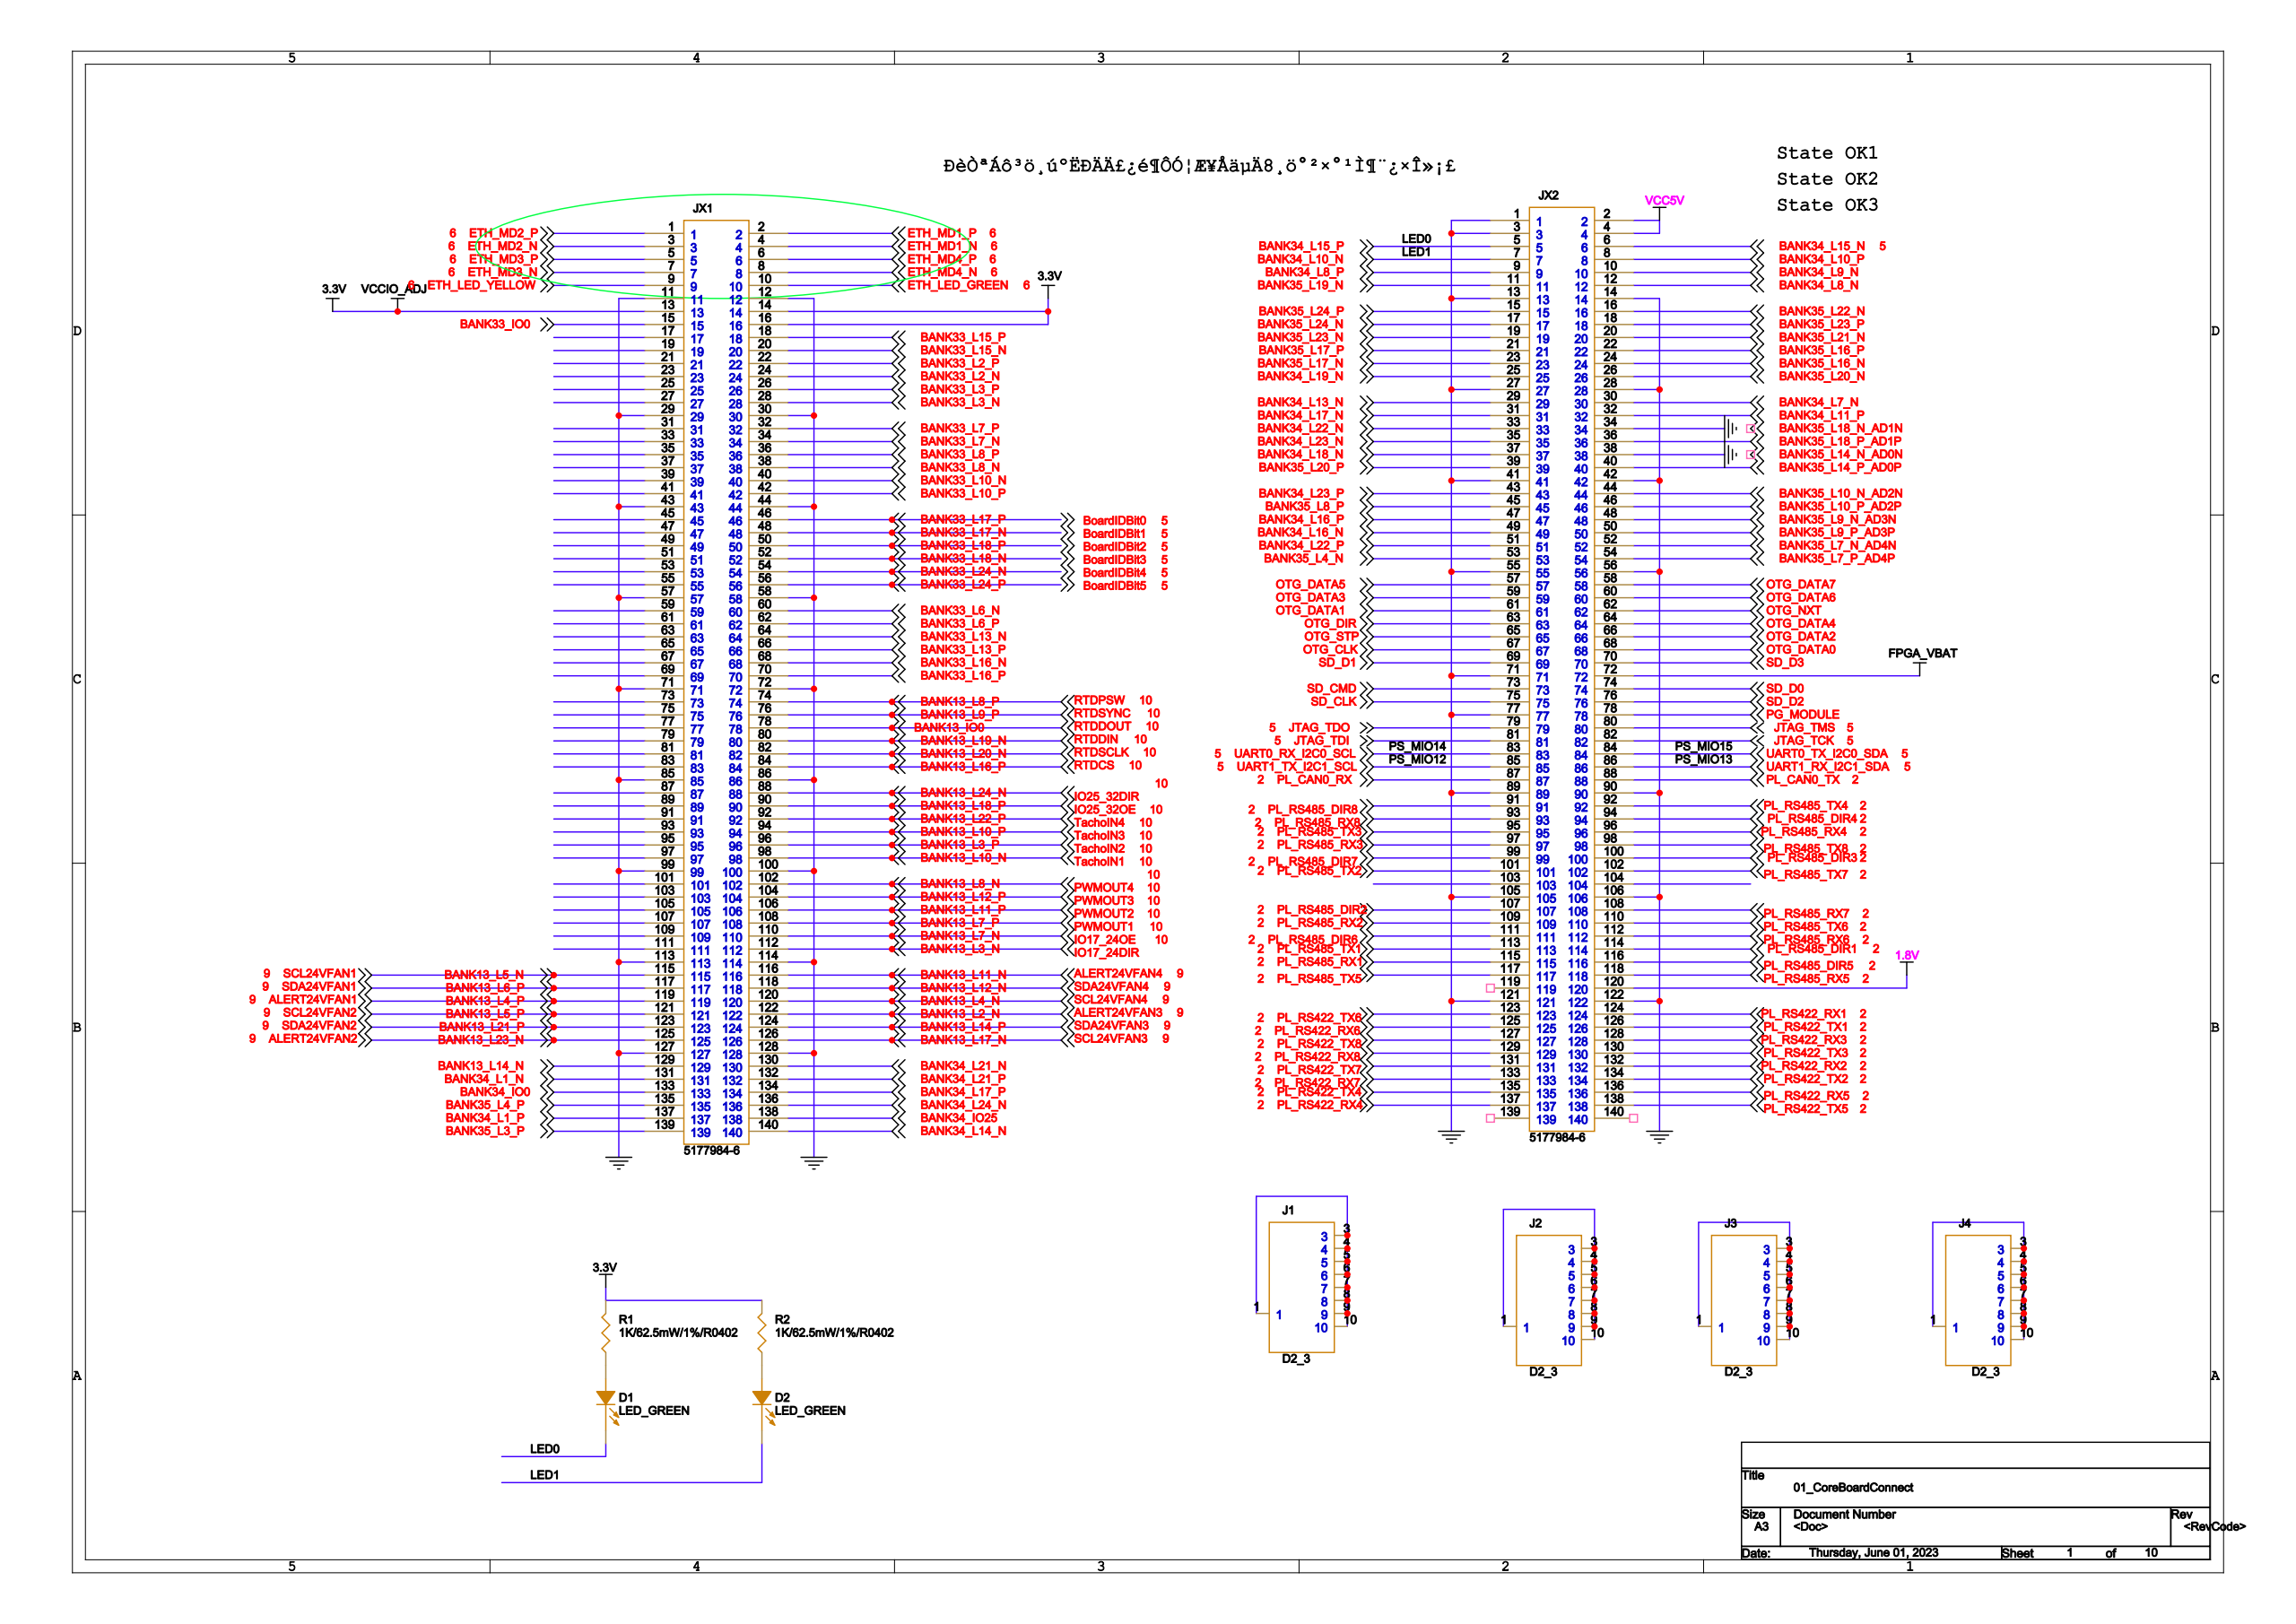Circuit board | Cadence Allegro | 480 parts | 625 nets | one sheet of the schematic
Parts on this sheet (reference | value | footprint):
D1 | LED_GREEN | LED0805
D2 | LED_GREEN | LED0805
J1 | D2_3 | D2_3
J2 | D2_3 | D2_3
J3 | D2_3 | D2_3
J4 | D2_3 | D2_3
JX1 | 5177984-6 | 5177983-6
JX2 | 5177984-6 | 5177983-6
R1 | 1K/62.5mW/1%/R0402 | 0402
R2 | 1K/62.5mW/1%/R0402 | 0402
Nets of these parts (net: part-pin ...):
ETH_MD2_P: JX1-1
ETH_LED_GREEN: JX1-10
BANK13_L8_N: JX1-102
BANK13_L12_P: JX1-104
BANK13_L11_P: JX1-106
BANK13_L7_P: JX1-108
BANK13_L7_N: JX1-110
BANK13_L3_N: JX1-112
BANK13_L5_N: JX1-115
ALERT24VFAN4: JX1-116
BANK13_L6_P: JX1-117
BANK13_L12_N: JX1-118
ALERT24VFAN1: JX1-119
BANK13_L4_N: JX1-120
BANK13_L5_P: JX1-121
ALERT24VFAN3: JX1-122
BANK13_L21_P: JX1-123
BANK13_L14_P: JX1-124
ALERT24VFAN2: JX1-125
BANK13_L17_N: JX1-126
BANK13_L14_N: JX1-129
3.3V: R1-2 R2-2 JX1-13 JX1-14 JX1-16
BANK34_L21_N: JX1-130
BANK34_L1_N: JX1-131
BANK34_L21_P: JX1-132
BANK34_IO0: JX1-133
BANK34_L17_P: JX1-134
BANK35_L4_P: JX1-135
BANK34_L24_N: JX1-136
BANK34_L1_P: JX1-137
BANK34_IO25: JX1-138
BANK35_L3_P: JX1-139
BANK34_L14_N: JX1-140
BANK33_IO0: JX1-15
BANK33_L15_P: JX1-18
ETH_MD1_P: JX1-2
BANK33_L15_N: JX1-20
BANK33_L2_P: JX1-22
BANK33_L2_N: JX1-24
BANK33_L3_P: JX1-26
BANK33_L3_N: JX1-28
ETH_MD2_N: JX1-3
BANK33_L7_P: JX1-32
BANK33_L7_N: JX1-34
BANK33_L8_P: JX1-36
BANK33_L8_N: JX1-38
ETH_MD1_N: JX1-4
BANK33_L10_N: JX1-40
BANK33_L10_P: JX1-42
BANK33_L17_P: JX1-46
BANK33_L17_N: JX1-48
ETH_MD3_P: JX1-5
BANK33_L18_P: JX1-50
BANK33_L18_N: JX1-52
BANK33_L24_N: JX1-54
BANK33_L24_P: JX1-56
ETH_MD4_P: JX1-6
BANK33_L6_N: JX1-60
BANK33_L6_P: JX1-62
BANK33_L13_N: JX1-64
BANK33_L13_P: JX1-66
BANK33_L16_N: JX1-68
ETH_MD3_N: JX1-7
BANK33_L16_P: JX1-70
BANK13_L8_P: JX1-74
BANK13_L9_P: JX1-76
BANK13_IO0: JX1-78
ETH_MD4_N: JX1-8
BANK13_L19_N: JX1-80
BANK13_L20_N: JX1-82
BANK13_L16_P: JX1-84
BANK13_L24_N: JX1-88
ETH_LED_YELLOW: JX1-9
BANK13_L18_P: JX1-90
BANK13_L22_P: JX1-92
BANK13_L10_P: JX1-94
BANK13_L3_P: JX1-96
BANK13_L10_N: JX1-98
BANK34_L9_N: JX2-10
PL_RS485_DIR3: JX2-100
PL_RS485_TX2: JX2-101
PL_RS485_TX7: JX2-102
PL_RS485_DIR2: JX2-107
PL_RS485_RX7: JX2-108
PL_RS485_RX2: JX2-109
BANK35_L19_N: JX2-11
PL_RS485_TX6: JX2-110
PL_RS485_DIR6: JX2-111
PL_RS485_RX6: JX2-112
PL_RS485_TX1: JX2-113
PL_RS485_DIR1: JX2-114
PL_RS485_RX1: JX2-115
PL_RS485_DIR5: JX2-116
PL_RS485_TX5: JX2-117
PL_RS485_RX5: JX2-118
BANK34_L8_N: JX2-12
1.8V: JX2-120
PL_RS422_TX6: JX2-123
PL_RS422_RX1: JX2-124
PL_RS422_RX6: JX2-125
PL_RS422_TX1: JX2-126
PL_RS422_TX8: JX2-127
PL_RS422_RX3: JX2-128
PL_RS422_RX8: JX2-129
PL_RS422_TX3: JX2-130
PL_RS422_TX7: JX2-131
PL_RS422_RX2: JX2-132
PL_RS422_RX7: JX2-133
PL_RS422_TX2: JX2-134
PL_RS422_TX4: JX2-135
PL_RS422_RX5: JX2-136
PL_RS422_RX4: JX2-137
PL_RS422_TX5: JX2-138
BANK35_L24_P: JX2-15
BANK35_L22_N: JX2-16
BANK35_L24_N: JX2-17
BANK35_L23_P: JX2-18
BANK35_L23_N: JX2-19
VCC5V: JX2-2 JX2-4
BANK35_L21_N: JX2-20
BANK35_L17_P: JX2-21
BANK35_L16_P: JX2-22
BANK35_L17_N: JX2-23
BANK35_L16_N: JX2-24
BANK34_L19_N: JX2-25
BANK35_L20_N: JX2-26
BANK34_L13_N: JX2-29
BANK34_L7_N: JX2-30
BANK34_L17_N: JX2-31
BANK34_L11_P: JX2-32
BANK34_L22_N: JX2-33
BANK34_L23_N: JX2-35
BANK35_L18_P_AD1P: JX2-36
BANK34_L18_N: JX2-37
BANK35_L20_P: JX2-39
BANK35_L14_P_AD0P: JX2-40
BANK34_L23_P: JX2-43
BANK35_L10_N_AD2N: JX2-44
BANK35_L8_P: JX2-45
BANK35_L10_P_AD2P: JX2-46
BANK34_L16_P: JX2-47
BANK35_L9_N_AD3N: JX2-48
BANK34_L16_N: JX2-49
BANK34_L15_P: D1-2 JX2-5
BANK35_L9_P_AD3P: JX2-50
BANK34_L22_P: JX2-51
BANK35_L7_N_AD4N: JX2-52
BANK35_L4_N: JX2-53
BANK35_L7_P_AD4P: JX2-54
OTG_DATA5: JX2-57
OTG_DATA7: JX2-58
OTG_DATA3: JX2-59
BANK34_L15_N: JX2-6
OTG_DATA6: JX2-60
OTG_DATA1: JX2-61
OTG_NXT: JX2-62
OTG_DIR: JX2-63
OTG_DATA4: JX2-64
OTG_STP: JX2-65
OTG_DATA2: JX2-66
OTG_CLK: JX2-67
OTG_DATA0: JX2-68
SD_D1: JX2-69
BANK34_L10_N: D2-2 JX2-7
SD_D3: JX2-70
FPGA_VBAT: JX2-72
SD_CMD: JX2-73
SD_D0: JX2-74
SD_CLK: JX2-75
SD_D2: JX2-76
PG_MODULE: JX2-78
JTAG_TDO: JX2-79
BANK34_L10_P: JX2-8
JTAG_TMS: JX2-80
JTAG_TDI: JX2-81
JTAG_TCK: JX2-82
UART0_RX_I2C0_SCL: JX2-83
UART0_TX_I2C0_SDA: JX2-84
UART1_TX_I2C1_SCL: JX2-85
UART1_RX_I2C1_SDA: JX2-86
PL_CAN0_RX: JX2-87
PL_CAN0_TX: JX2-88
BANK34_L8_P: JX2-9
PL_RS485_DIR8: JX2-91
PL_RS485_TX4: JX2-92
PL_RS485_RX8: JX2-93
PL_RS485_DIR4: JX2-94
PL_RS485_TX3: JX2-95
PL_RS485_RX4: JX2-96
PL_RS485_RX3: JX2-97
PL_RS485_TX8: JX2-98
PL_RS485_DIR7: JX2-99
N231084320: D1-1 R1-1
N231087860: D2-1 R2-1
N23884939: J1-1 J1-3 J1-4 J1-5 J1-6 J1-7 J1-8 J1-9 J1-10
N23884945: J2-1 J2-3 J2-4 J2-5 J2-6 J2-7 J2-8 J2-9 J2-10
N23884981: J3-1 J3-3 J3-4 J3-5 J3-6 J3-7 J3-8 J3-9 J3-10
N23884987: J4-1 J4-3 J4-4 J4-5 J4-6 J4-7 J4-8 J4-9 J4-10